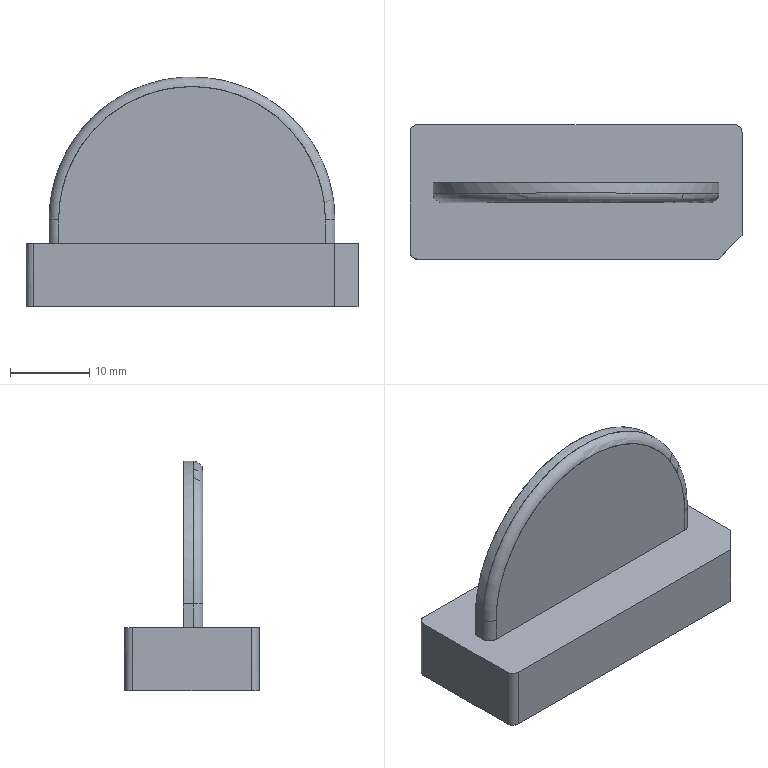CAM job | PowerMill | 3-axis milling, other | part box 42 x 17 x 29.081 mm
Tools:
number,name,type,diameter,tip_radius,length,cutting_length,overhang,flutes,holder,toolpaths_using
1,D10C,end_mill,10.0,0.0,60.0,,30.0,1,D42L35,1
1,D10C_1_1_1,end_mill,10.0,0.0,60.0,,29.52,1,D42L35,3
2,D4C_1_1,end_mill,4.0,0.0,30.0,,21.08,1,D42L35,2
3,D10_1_1_1,end_mill,10.0,0.0,60.0,,29.24,1,D42L35,2
7,R2_1_1,ball_nosed,4.0,2.0,30.0,,20.4,1,D42L35,1
14,D4_1_1,end_mill,4.0,0.0,30.0,,21.36,1,D42L35,1
13,Text_D4_1_1,taper_spherical,4.0,0.3,60.0,,21.36,1,D42L35,1
Operations:
program,toolpath,strategy,tool,tool_number,tool_diameter,tip_radius,flutes,spindle_rpm,feed_cut,surface_speed_m_min_computed,feed_per_tooth_computed,tolerance,thickness,stepover,stepdown,cut_length,cut_time_min,total_time_min,workplane
02-B01-8-F,精公开粗01-扫面平行-D10C,raster_area_clear,D10C_1_1_1,1,10.0,0.0,1.0,8000.0,10000.0,251.33,1.25,0.03,0.28,6.0,1.0,260.36,0.026,0.0323,
02-B01-8-F,精公开粗01-外形偏置-D10C,offset_area_clear,D10C_1_1_1,1,10.0,0.0,1.0,8000.0,10000.0,251.33,1.25,0.03,0.28,6.0,1.0,14004.708,1.401,1.531,
02-B01-8-F,精公开粗01-基准台等高-D10C,constantz,D10C_1_1_1,1,10.0,0.0,1.0,8000.0,10000.0,251.33,1.25,0.03,0.07,5.0,0.4,3229.058,0.323,0.3348,
02-B01-8-F,精公再粗02-外形偏置-D4C,offset_area_clear,D4C_1_1,2,4.0,0.0,1.0,18000.0,6000.0,226.19,0.3333,0.03,0.0,2.0,1.0,8015.574,1.336,1.376,
02-B01-8-F,精公再粗02-平行中光-D4C,raster,D4C_1_1,2,4.0,0.0,1.0,18000.0,6000.0,226.19,0.3333,0.03,0.0,0.2,1.0,1845.162,0.307,0.3257,
02-B01-8-F,精公基准台01-基准面偏置-D10,offset_area_clear,D10_1_1_1,3,10.0,0.0,1.0,8500.0,600.0,267.04,0.0706,0.005,0.38,5.0,1.0,118.711,0.198,0.2194,
02-B01-8-F,精公基准台01-基准台侧光-D10,profile_area_clear,D10_1_1_1,3,10.0,0.0,1.0,8500.0,600.0,267.04,0.0706,0.005,0.0,0.08,1.0,293.234,0.489,0.5552,
02-B01-8-F,精公精光01-平行-R2,raster,R2_1_1,7,4.0,2.0,1.0,18000.0,2000.0,226.19,0.1111,0.005,-0.075,0.05,1.0,8004.004,4.002,4.086,
02-B01-8-F,精公精光02-等高-D4,constantz,D4_1_1,14,4.0,0.0,1.0,18000.0,2000.0,226.19,0.1111,0.005,-0.075,5.0,0.06,26410.792,13.205,13.79,
02-B01-8-F,精公刻字01-刻字-Text_D4,pattern,Text_D4_1_1,13,4.0,0.3,1.0,15000.0,1000.0,188.5,0.0667,0.005,0.0,5.0,1.0,78.59,0.079,0.1093,
,精公开粗01-外形偏置-D10C_Reference,offset_area_clear,D10C,1,10.0,0.0,1.0,8000.0,10000.0,251.33,1.25,0.03,0.28,6.0,1.0,27821.925,2.782,3.039,